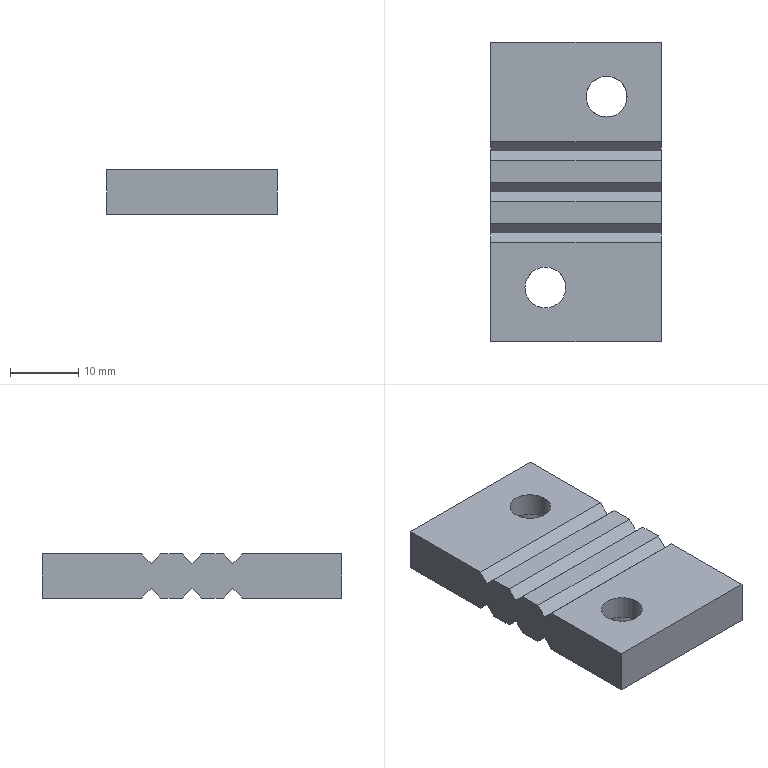Part | NX | features DATUM_CSYS 6, SKETCH 5, EXTRUDE 3, DATUM_PLANE 2, EXTRACT_STRING 2, SWP104 2, BREP 1, Instance Feature 1, Mirror Feature 1, TRIM BODY 1, UNITE 1 | 1 solid | 28 faces | box 25 x 44 x 6.5 mm | volume 6256 mm3 | plane 24 | cylinder 2 | cone 2 | commonest cylinder face diameters 6 x2
STEP:
#1=CARTESIAN_POINT('',(12.5,4.586,0.));
#2=VERTEX_POINT('',#1);
#3=CARTESIAN_POINT('',(12.5,6.,-1.414));
#4=VERTEX_POINT('',#3);
#5=CARTESIAN_POINT('',(12.5,-11.957,16.543));
#6=DIRECTION('',(0.,0.7071,-0.7071));
#7=VECTOR('',#6,1000.);
#8=LINE('',#5,#7);
#9=EDGE_CURVE('',#2,#4,#8,.T.);
#10=ORIENTED_EDGE('',*,*,#9,.F.);
#11=CARTESIAN_POINT('',(12.5,1.414,0.));
#12=VERTEX_POINT('',#11);
#13=CARTESIAN_POINT('',(12.5,-22.,0.));
#14=DIRECTION('',(0.,1.,0.));
#15=VECTOR('',#14,1000.);
#16=LINE('',#13,#15);
#17=EDGE_CURVE('',#12,#2,#16,.T.);
#18=ORIENTED_EDGE('',*,*,#17,.F.);
#19=CARTESIAN_POINT('',(12.5,0.,-1.414));
#20=VERTEX_POINT('',#19);
#21=CARTESIAN_POINT('',(12.5,-7.043,-8.457));
#22=DIRECTION('',(0.,0.7071,0.7071));
#23=VECTOR('',#22,1000.);
#24=LINE('',#21,#23);
#25=EDGE_CURVE('',#20,#12,#24,.T.);
#26=ORIENTED_EDGE('',*,*,#25,.F.);
#27=CARTESIAN_POINT('',(12.5,-1.414,0.));
#28=VERTEX_POINT('',#27);
#29=CARTESIAN_POINT('',(12.5,-14.957,13.543));
#30=DIRECTION('',(0.,0.7071,-0.7071));
#31=VECTOR('',#30,1000.);
#32=LINE('',#29,#31);
#33=EDGE_CURVE('',#28,#20,#32,.T.);
#34=ORIENTED_EDGE('',*,*,#33,.F.);
#35=CARTESIAN_POINT('',(12.5,-4.586,0.));
#36=VERTEX_POINT('',#35);
#37=CARTESIAN_POINT('',(12.5,-22.,0.));
#38=DIRECTION('',(0.,1.,0.));
#39=VECTOR('',#38,1000.);
#40=LINE('',#37,#39);
#41=EDGE_CURVE('',#36,#28,#40,.T.);
#42=ORIENTED_EDGE('',*,*,#41,.F.);
#43=CARTESIAN_POINT('',(12.5,-6.,-1.414));
#44=VERTEX_POINT('',#43);
#45=CARTESIAN_POINT('',(12.5,-10.043,-5.457));
#46=DIRECTION('',(0.,0.7071,0.7071));
#47=VECTOR('',#46,1000.);
#48=LINE('',#45,#47);
#49=EDGE_CURVE('',#44,#36,#48,.T.);
#50=ORIENTED_EDGE('',*,*,#49,.F.);
#51=CARTESIAN_POINT('',(12.5,-7.414,0.));
#52=VERTEX_POINT('',#51);
#53=CARTESIAN_POINT('',(12.5,-17.957,10.543));
#54=DIRECTION('',(0.,0.7071,-0.7071));
#55=VECTOR('',#54,1000.);
#56=LINE('',#53,#55);
#57=EDGE_CURVE('',#52,#44,#56,.T.);
#58=ORIENTED_EDGE('',*,*,#57,.F.);
#59=CARTESIAN_POINT('',(12.5,-22.,0.));
#60=VERTEX_POINT('',#59);
#61=CARTESIAN_POINT('',(12.5,-22.,0.));
#62=DIRECTION('',(0.,1.,0.));
#63=VECTOR('',#62,1000.);
#64=LINE('',#61,#63);
#65=EDGE_CURVE('',#60,#52,#64,.T.);
#66=ORIENTED_EDGE('',*,*,#65,.F.);
#67=CARTESIAN_POINT('',(12.5,-22.,-6.5));
#68=VERTEX_POINT('',#67);
#69=CARTESIAN_POINT('',(12.5,-22.,6.5));
#70=DIRECTION('',(0.,0.,-1.));
#71=VECTOR('',#70,1000.);
#72=LINE('',#69,#71);
#73=EDGE_CURVE('',#60,#68,#72,.T.);
#74=ORIENTED_EDGE('',*,*,#73,.T.);
#75=CARTESIAN_POINT('',(12.5,-7.414,-6.5));
#76=VERTEX_POINT('',#75);
#77=CARTESIAN_POINT('',(12.5,-22.,-6.5));
#78=DIRECTION('',(0.,1.,0.));
#79=VECTOR('',#78,1000.);
#80=LINE('',#77,#79);
#81=EDGE_CURVE('',#68,#76,#80,.T.);
#82=ORIENTED_EDGE('',*,*,#81,.T.);
#83=CARTESIAN_POINT('',(12.5,-6.,-5.086));
#84=VERTEX_POINT('',#83);
#85=CARTESIAN_POINT('',(12.5,-8.207,-7.293));
#86=DIRECTION('',(0.,0.7071,0.7071));
#87=VECTOR('',#86,1000.);
#88=LINE('',#85,#87);
#89=EDGE_CURVE('',#76,#84,#88,.T.);
#90=ORIENTED_EDGE('',*,*,#89,.T.);
#91=CARTESIAN_POINT('',(12.5,-4.586,-6.5));
#92=VERTEX_POINT('',#91);
#93=CARTESIAN_POINT('',(12.5,-19.793,8.707));
#94=DIRECTION('',(0.,0.7071,-0.7071));
#95=VECTOR('',#94,1000.);
#96=LINE('',#93,#95);
#97=EDGE_CURVE('',#84,#92,#96,.T.);
#98=ORIENTED_EDGE('',*,*,#97,.T.);
#99=CARTESIAN_POINT('',(12.5,-1.414,-6.5));
#100=VERTEX_POINT('',#99);
#101=CARTESIAN_POINT('',(12.5,-22.,-6.5));
#102=DIRECTION('',(0.,1.,0.));
#103=VECTOR('',#102,1000.);
#104=LINE('',#101,#103);
#105=EDGE_CURVE('',#92,#100,#104,.T.);
#106=ORIENTED_EDGE('',*,*,#105,.T.);
#107=CARTESIAN_POINT('',(12.5,0.,-5.086));
#108=VERTEX_POINT('',#107);
#109=CARTESIAN_POINT('',(12.5,-5.207,-10.293));
#110=DIRECTION('',(0.,0.7071,0.7071));
#111=VECTOR('',#110,1000.);
#112=LINE('',#109,#111);
#113=EDGE_CURVE('',#100,#108,#112,.T.);
#114=ORIENTED_EDGE('',*,*,#113,.T.);
#115=CARTESIAN_POINT('',(12.5,1.414,-6.5));
#116=VERTEX_POINT('',#115);
#117=CARTESIAN_POINT('',(12.5,-16.793,11.707));
#118=DIRECTION('',(0.,0.7071,-0.7071));
#119=VECTOR('',#118,1000.);
#120=LINE('',#117,#119);
#121=EDGE_CURVE('',#108,#116,#120,.T.);
#122=ORIENTED_EDGE('',*,*,#121,.T.);
#123=CARTESIAN_POINT('',(12.5,4.586,-6.5));
#124=VERTEX_POINT('',#123);
#125=CARTESIAN_POINT('',(12.5,-22.,-6.5));
#126=DIRECTION('',(0.,1.,0.));
#127=VECTOR('',#126,1000.);
#128=LINE('',#125,#127);
#129=EDGE_CURVE('',#116,#124,#128,.T.);
#130=ORIENTED_EDGE('',*,*,#129,.T.);
#131=CARTESIAN_POINT('',(12.5,6.,-5.086));
#132=VERTEX_POINT('',#131);
#133=CARTESIAN_POINT('',(12.5,-2.207,-13.293));
#134=DIRECTION('',(0.,0.7071,0.7071));
#135=VECTOR('',#134,1000.);
#136=LINE('',#133,#135);
#137=EDGE_CURVE('',#124,#132,#136,.T.);
#138=ORIENTED_EDGE('',*,*,#137,.T.);
#139=CARTESIAN_POINT('',(12.5,7.414,-6.5));
#140=VERTEX_POINT('',#139);
#141=CARTESIAN_POINT('',(12.5,-13.793,14.707));
#142=DIRECTION('',(0.,0.7071,-0.7071));
#143=VECTOR('',#142,1000.);
#144=LINE('',#141,#143);
#145=EDGE_CURVE('',#132,#140,#144,.T.);
#146=ORIENTED_EDGE('',*,*,#145,.T.);
#147=CARTESIAN_POINT('',(12.5,22.,-6.5));
#148=VERTEX_POINT('',#147);
#149=CARTESIAN_POINT('',(12.5,-22.,-6.5));
#150=DIRECTION('',(0.,1.,0.));
#151=VECTOR('',#150,1000.);
#152=LINE('',#149,#151);
#153=EDGE_CURVE('',#140,#148,#152,.T.);
#154=ORIENTED_EDGE('',*,*,#153,.T.);
#155=CARTESIAN_POINT('',(12.5,22.,0.));
#156=VERTEX_POINT('',#155);
#157=CARTESIAN_POINT('',(12.5,22.,6.5));
#158=DIRECTION('',(0.,0.,-1.));
#159=VECTOR('',#158,1000.);
#160=LINE('',#157,#159);
#161=EDGE_CURVE('',#156,#148,#160,.T.);
#162=ORIENTED_EDGE('',*,*,#161,.F.);
#163=CARTESIAN_POINT('',(12.5,7.414,0.));
#164=VERTEX_POINT('',#163);
#165=CARTESIAN_POINT('',(12.5,-22.,0.));
#166=DIRECTION('',(0.,1.,0.));
#167=VECTOR('',#166,1000.);
#168=LINE('',#165,#167);
#169=EDGE_CURVE('',#164,#156,#168,.T.);
#170=ORIENTED_EDGE('',*,*,#169,.F.);
#171=CARTESIAN_POINT('',(12.5,-4.043,-11.457));
#172=DIRECTION('',(0.,0.7071,0.7071));
#173=VECTOR('',#172,1000.);
#174=LINE('',#171,#173);
#175=EDGE_CURVE('',#4,#164,#174,.T.);
#176=ORIENTED_EDGE('',*,*,#175,.F.);
#177=EDGE_LOOP('',(#10,#18,#26,#34,#42,#50,#58,#66,#74,#82,#90,#98,#106,#114,#122,#130,#138,#146,#154,#162,#170,#176));
#178=FACE_BOUND('',#177,.T.);
#179=CARTESIAN_POINT('',(12.5,-22.,6.5));
#180=DIRECTION('',(-1.,0.,0.));
#181=DIRECTION('',(0.,0.,1.));
#182=AXIS2_PLACEMENT_3D('',#179,#180,#181);
#183=PLANE('',#182);
#184=ADVANCED_FACE('',(#178),#183,.F.);
#185=ORIENTED_EDGE('',*,*,#17,.T.);
#186=CARTESIAN_POINT('',(-12.5,4.586,0.));
#187=VERTEX_POINT('',#186);
#188=CARTESIAN_POINT('',(19.5,4.586,0.));
#189=DIRECTION('',(-1.,0.,0.));
#190=VECTOR('',#189,1000.);
#191=LINE('',#188,#190);
#192=EDGE_CURVE('',#2,#187,#191,.T.);
#193=ORIENTED_EDGE('',*,*,#192,.T.);
#194=CARTESIAN_POINT('',(-12.5,1.414,0.));
#195=VERTEX_POINT('',#194);
#196=CARTESIAN_POINT('',(-12.5,22.,0.));
#197=DIRECTION('',(0.,-1.,0.));
#198=VECTOR('',#197,1000.);
#199=LINE('',#196,#198);
#200=EDGE_CURVE('',#187,#195,#199,.T.);
#201=ORIENTED_EDGE('',*,*,#200,.T.);
#202=CARTESIAN_POINT('',(19.5,1.414,0.));
#203=DIRECTION('',(-1.,0.,0.));
#204=VECTOR('',#203,1000.);
#205=LINE('',#202,#204);
#206=EDGE_CURVE('',#12,#195,#205,.T.);
#207=ORIENTED_EDGE('',*,*,#206,.F.);
#208=EDGE_LOOP('',(#185,#193,#201,#207));
#209=FACE_BOUND('',#208,.T.);
#210=CARTESIAN_POINT('',(0.,0.,0.));
#211=DIRECTION('',(0.,0.,1.));
#212=DIRECTION('',(1.,0.,0.));
#213=AXIS2_PLACEMENT_3D('',#210,#211,#212);
#214=PLANE('',#213);
#215=ADVANCED_FACE('',(#209),#214,.T.);
#216=CARTESIAN_POINT('',(7.5,14.,0.));
#217=VERTEX_POINT('',#216);
#218=CARTESIAN_POINT('',(4.5,14.,0.));
#219=DIRECTION('',(0.,0.,1.));
#220=DIRECTION('',(1.,0.,0.));
#221=AXIS2_PLACEMENT_3D('',#218,#219,#220);
#222=CIRCLE('',#221,3.);
#223=EDGE_CURVE('',#217,#217,#222,.F.);
#224=ORIENTED_EDGE('',*,*,#223,.T.);
#225=EDGE_LOOP('',(#224));
#226=FACE_BOUND('',#225,.T.);
#227=CARTESIAN_POINT('',(-12.5,22.,0.));
#228=VERTEX_POINT('',#227);
#229=CARTESIAN_POINT('',(-12.5,7.414,0.));
#230=VERTEX_POINT('',#229);
#231=CARTESIAN_POINT('',(-12.5,22.,0.));
#232=DIRECTION('',(0.,-1.,0.));
#233=VECTOR('',#232,1000.);
#234=LINE('',#231,#233);
#235=EDGE_CURVE('',#228,#230,#234,.T.);
#236=ORIENTED_EDGE('',*,*,#235,.T.);
#237=CARTESIAN_POINT('',(19.5,7.414,0.));
#238=DIRECTION('',(-1.,0.,0.));
#239=VECTOR('',#238,1000.);
#240=LINE('',#237,#239);
#241=EDGE_CURVE('',#164,#230,#240,.T.);
#242=ORIENTED_EDGE('',*,*,#241,.F.);
#243=ORIENTED_EDGE('',*,*,#169,.T.);
#244=CARTESIAN_POINT('',(12.5,22.,0.));
#245=DIRECTION('',(-1.,0.,0.));
#246=VECTOR('',#245,1000.);
#247=LINE('',#244,#246);
#248=EDGE_CURVE('',#156,#228,#247,.T.);
#249=ORIENTED_EDGE('',*,*,#248,.T.);
#250=EDGE_LOOP('',(#236,#242,#243,#249));
#251=FACE_BOUND('',#250,.T.);
#252=CARTESIAN_POINT('',(0.,0.,0.));
#253=DIRECTION('',(0.,0.,1.));
#254=DIRECTION('',(1.,0.,0.));
#255=AXIS2_PLACEMENT_3D('',#252,#253,#254);
#256=PLANE('',#255);
#257=ADVANCED_FACE('',(#226,#251),#256,.T.);
#258=ORIENTED_EDGE('',*,*,#41,.T.);
#259=CARTESIAN_POINT('',(-12.5,-1.414,0.));
#260=VERTEX_POINT('',#259);
#261=CARTESIAN_POINT('',(19.5,-1.414,0.));
#262=DIRECTION('',(-1.,0.,0.));
#263=VECTOR('',#262,1000.);
#264=LINE('',#261,#263);
#265=EDGE_CURVE('',#28,#260,#264,.T.);
#266=ORIENTED_EDGE('',*,*,#265,.T.);
#267=CARTESIAN_POINT('',(-12.5,-4.586,0.));
#268=VERTEX_POINT('',#267);
#269=CARTESIAN_POINT('',(-12.5,22.,0.));
#270=DIRECTION('',(0.,-1.,0.));
#271=VECTOR('',#270,1000.);
#272=LINE('',#269,#271);
#273=EDGE_CURVE('',#260,#268,#272,.T.);
#274=ORIENTED_EDGE('',*,*,#273,.T.);
#275=CARTESIAN_POINT('',(19.5,-4.586,0.));
#276=DIRECTION('',(-1.,0.,0.));
#277=VECTOR('',#276,1000.);
#278=LINE('',#275,#277);
#279=EDGE_CURVE('',#36,#268,#278,.T.);
#280=ORIENTED_EDGE('',*,*,#279,.F.);
#281=EDGE_LOOP('',(#258,#266,#274,#280));
#282=FACE_BOUND('',#281,.T.);
#283=CARTESIAN_POINT('',(0.,0.,0.));
#284=DIRECTION('',(0.,0.,1.));
#285=DIRECTION('',(1.,0.,0.));
#286=AXIS2_PLACEMENT_3D('',#283,#284,#285);
#287=PLANE('',#286);
#288=ADVANCED_FACE('',(#282),#287,.T.);
#289=CARTESIAN_POINT('',(-1.5,-14.043,0.));
#290=VERTEX_POINT('',#289);
#291=CARTESIAN_POINT('',(-4.5,-14.043,0.));
#292=DIRECTION('',(0.,0.,1.));
#293=DIRECTION('',(1.,0.,0.));
#294=AXIS2_PLACEMENT_3D('',#291,#292,#293);
#295=CIRCLE('',#294,3.);
#296=EDGE_CURVE('',#290,#290,#295,.T.);
#297=ORIENTED_EDGE('',*,*,#296,.F.);
#298=EDGE_LOOP('',(#297));
#299=FACE_BOUND('',#298,.T.);
#300=ORIENTED_EDGE('',*,*,#65,.T.);
#301=CARTESIAN_POINT('',(-12.5,-7.414,0.));
#302=VERTEX_POINT('',#301);
#303=CARTESIAN_POINT('',(19.5,-7.414,0.));
#304=DIRECTION('',(-1.,0.,0.));
#305=VECTOR('',#304,1000.);
#306=LINE('',#303,#305);
#307=EDGE_CURVE('',#52,#302,#306,.T.);
#308=ORIENTED_EDGE('',*,*,#307,.T.);
#309=CARTESIAN_POINT('',(-12.5,-22.,0.));
#310=VERTEX_POINT('',#309);
#311=CARTESIAN_POINT('',(-12.5,22.,0.));
#312=DIRECTION('',(0.,-1.,0.));
#313=VECTOR('',#312,1000.);
#314=LINE('',#311,#313);
#315=EDGE_CURVE('',#302,#310,#314,.T.);
#316=ORIENTED_EDGE('',*,*,#315,.T.);
#317=CARTESIAN_POINT('',(-12.5,-22.,0.));
#318=DIRECTION('',(1.,0.,0.));
#319=VECTOR('',#318,1000.);
#320=LINE('',#317,#319);
#321=EDGE_CURVE('',#310,#60,#320,.T.);
#322=ORIENTED_EDGE('',*,*,#321,.T.);
#323=EDGE_LOOP('',(#300,#308,#316,#322));
#324=FACE_BOUND('',#323,.T.);
#325=CARTESIAN_POINT('',(0.,0.,0.));
#326=DIRECTION('',(0.,0.,1.));
#327=DIRECTION('',(1.,0.,0.));
#328=AXIS2_PLACEMENT_3D('',#325,#326,#327);
#329=PLANE('',#328);
#330=ADVANCED_FACE('',(#299,#324),#329,.T.);
#331=CARTESIAN_POINT('',(-12.5,6.,-1.414));
#332=VERTEX_POINT('',#331);
#333=CARTESIAN_POINT('',(-12.5,4.586,0.));
#334=DIRECTION('',(0.,0.7071,-0.7071));
#335=VECTOR('',#334,1000.);
#336=LINE('',#333,#335);
#337=EDGE_CURVE('',#187,#332,#336,.T.);
#338=ORIENTED_EDGE('',*,*,#337,.T.);
#339=CARTESIAN_POINT('',(-12.5,6.,-1.414));
#340=DIRECTION('',(0.,0.7071,0.7071));
#341=VECTOR('',#340,1000.);
#342=LINE('',#339,#341);
#343=EDGE_CURVE('',#332,#230,#342,.T.);
#344=ORIENTED_EDGE('',*,*,#343,.T.);
#345=ORIENTED_EDGE('',*,*,#235,.F.);
#346=CARTESIAN_POINT('',(-12.5,22.,-6.5));
#347=VERTEX_POINT('',#346);
#348=CARTESIAN_POINT('',(-12.5,22.,6.5));
#349=DIRECTION('',(0.,0.,-1.));
#350=VECTOR('',#349,1000.);
#351=LINE('',#348,#350);
#352=EDGE_CURVE('',#228,#347,#351,.T.);
#353=ORIENTED_EDGE('',*,*,#352,.T.);
#354=CARTESIAN_POINT('',(-12.5,7.414,-6.5));
#355=VERTEX_POINT('',#354);
#356=CARTESIAN_POINT('',(-12.5,22.,-6.5));
#357=DIRECTION('',(0.,-1.,0.));
#358=VECTOR('',#357,1000.);
#359=LINE('',#356,#358);
#360=EDGE_CURVE('',#347,#355,#359,.T.);
#361=ORIENTED_EDGE('',*,*,#360,.T.);
#362=CARTESIAN_POINT('',(-12.5,6.,-5.086));
#363=VERTEX_POINT('',#362);
#364=CARTESIAN_POINT('',(-12.5,6.,-5.086));
#365=DIRECTION('',(0.,0.7071,-0.7071));
#366=VECTOR('',#365,1000.);
#367=LINE('',#364,#366);
#368=EDGE_CURVE('',#363,#355,#367,.T.);
#369=ORIENTED_EDGE('',*,*,#368,.F.);
#370=CARTESIAN_POINT('',(-12.5,4.586,-6.5));
#371=VERTEX_POINT('',#370);
#372=CARTESIAN_POINT('',(-12.5,4.586,-6.5));
#373=DIRECTION('',(0.,0.7071,0.7071));
#374=VECTOR('',#373,1000.);
#375=LINE('',#372,#374);
#376=EDGE_CURVE('',#371,#363,#375,.T.);
#377=ORIENTED_EDGE('',*,*,#376,.F.);
#378=CARTESIAN_POINT('',(-12.5,1.414,-6.5));
#379=VERTEX_POINT('',#378);
#380=CARTESIAN_POINT('',(-12.5,22.,-6.5));
#381=DIRECTION('',(0.,-1.,0.));
#382=VECTOR('',#381,1000.);
#383=LINE('',#380,#382);
#384=EDGE_CURVE('',#371,#379,#383,.T.);
#385=ORIENTED_EDGE('',*,*,#384,.T.);
#386=CARTESIAN_POINT('',(-12.5,0.,-5.086));
#387=VERTEX_POINT('',#386);
#388=CARTESIAN_POINT('',(-12.5,0.,-5.086));
#389=DIRECTION('',(0.,0.7071,-0.7071));
#390=VECTOR('',#389,1000.);
#391=LINE('',#388,#390);
#392=EDGE_CURVE('',#387,#379,#391,.T.);
#393=ORIENTED_EDGE('',*,*,#392,.F.);
#394=CARTESIAN_POINT('',(-12.5,-1.414,-6.5));
#395=VERTEX_POINT('',#394);
#396=CARTESIAN_POINT('',(-12.5,-1.414,-6.5));
#397=DIRECTION('',(0.,0.7071,0.7071));
#398=VECTOR('',#397,1000.);
#399=LINE('',#396,#398);
#400=EDGE_CURVE('',#395,#387,#399,.T.);
#401=ORIENTED_EDGE('',*,*,#400,.F.);
#402=CARTESIAN_POINT('',(-12.5,-4.586,-6.5));
#403=VERTEX_POINT('',#402);
#404=CARTESIAN_POINT('',(-12.5,22.,-6.5));
#405=DIRECTION('',(0.,-1.,0.));
#406=VECTOR('',#405,1000.);
#407=LINE('',#404,#406);
#408=EDGE_CURVE('',#395,#403,#407,.T.);
#409=ORIENTED_EDGE('',*,*,#408,.T.);
#410=CARTESIAN_POINT('',(-12.5,-6.,-5.086));
#411=VERTEX_POINT('',#410);
#412=CARTESIAN_POINT('',(-12.5,-6.,-5.086));
#413=DIRECTION('',(0.,0.7071,-0.7071));
#414=VECTOR('',#413,1000.);
#415=LINE('',#412,#414);
#416=EDGE_CURVE('',#411,#403,#415,.T.);
#417=ORIENTED_EDGE('',*,*,#416,.F.);
#418=CARTESIAN_POINT('',(-12.5,-7.414,-6.5));
#419=VERTEX_POINT('',#418);
#420=CARTESIAN_POINT('',(-12.5,-7.414,-6.5));
#421=DIRECTION('',(0.,0.7071,0.7071));
#422=VECTOR('',#421,1000.);
#423=LINE('',#420,#422);
#424=EDGE_CURVE('',#419,#411,#423,.T.);
#425=ORIENTED_EDGE('',*,*,#424,.F.);
#426=CARTESIAN_POINT('',(-12.5,-22.,-6.5));
#427=VERTEX_POINT('',#426);
#428=CARTESIAN_POINT('',(-12.5,22.,-6.5));
#429=DIRECTION('',(0.,-1.,0.));
#430=VECTOR('',#429,1000.);
#431=LINE('',#428,#430);
#432=EDGE_CURVE('',#419,#427,#431,.T.);
#433=ORIENTED_EDGE('',*,*,#432,.T.);
#434=CARTESIAN_POINT('',(-12.5,-22.,6.5));
#435=DIRECTION('',(0.,0.,-1.));
#436=VECTOR('',#435,1000.);
#437=LINE('',#434,#436);
#438=EDGE_CURVE('',#310,#427,#437,.T.);
#439=ORIENTED_EDGE('',*,*,#438,.F.);
#440=ORIENTED_EDGE('',*,*,#315,.F.);
#441=CARTESIAN_POINT('',(-12.5,-6.,-1.414));
#442=VERTEX_POINT('',#441);
#443=CARTESIAN_POINT('',(-12.5,-7.414,0.));
#444=DIRECTION('',(0.,0.7071,-0.7071));
#445=VECTOR('',#444,1000.);
#446=LINE('',#443,#445);
#447=EDGE_CURVE('',#302,#442,#446,.T.);
#448=ORIENTED_EDGE('',*,*,#447,.T.);
#449=CARTESIAN_POINT('',(-12.5,-6.,-1.414));
#450=DIRECTION('',(0.,0.7071,0.7071));
#451=VECTOR('',#450,1000.);
#452=LINE('',#449,#451);
#453=EDGE_CURVE('',#442,#268,#452,.T.);
#454=ORIENTED_EDGE('',*,*,#453,.T.);
#455=ORIENTED_EDGE('',*,*,#273,.F.);
#456=CARTESIAN_POINT('',(-12.5,0.,-1.414));
#457=VERTEX_POINT('',#456);
#458=CARTESIAN_POINT('',(-12.5,-1.414,0.));
#459=DIRECTION('',(0.,0.7071,-0.7071));
#460=VECTOR('',#459,1000.);
#461=LINE('',#458,#460);
#462=EDGE_CURVE('',#260,#457,#461,.T.);
#463=ORIENTED_EDGE('',*,*,#462,.T.);
#464=CARTESIAN_POINT('',(-12.5,0.,-1.414));
#465=DIRECTION('',(0.,0.7071,0.7071));
#466=VECTOR('',#465,1000.);
#467=LINE('',#464,#466);
#468=EDGE_CURVE('',#457,#195,#467,.T.);
#469=ORIENTED_EDGE('',*,*,#468,.T.);
#470=ORIENTED_EDGE('',*,*,#200,.F.);
#471=EDGE_LOOP('',(#338,#344,#345,#353,#361,#369,#377,#385,#393,#401,#409,#417,#425,#433,#439,#440,#448,#454,#455,#463,#469,#470));
#472=FACE_BOUND('',#471,.T.);
#473=CARTESIAN_POINT('',(-12.5,22.,6.5));
#474=DIRECTION('',(1.,0.,0.));
#475=DIRECTION('',(0.,0.,-1.));
#476=AXIS2_PLACEMENT_3D('',#473,#474,#475);
#477=PLANE('',#476);
#478=ADVANCED_FACE('',(#472),#477,.F.);
#479=CARTESIAN_POINT('',(19.5,-7.414,-6.5));
#480=DIRECTION('',(-1.,0.,0.));
#481=VECTOR('',#480,1000.);
#482=LINE('',#479,#481);
#483=EDGE_CURVE('',#76,#419,#482,.T.);
#484=ORIENTED_EDGE('',*,*,#483,.F.);
#485=ORIENTED_EDGE('',*,*,#81,.F.);
#486=CARTESIAN_POINT('',(-12.5,-22.,-6.5));
#487=DIRECTION('',(1.,0.,0.));
#488=VECTOR('',#487,1000.);
#489=LINE('',#486,#488);
#490=EDGE_CURVE('',#427,#68,#489,.T.);
#491=ORIENTED_EDGE('',*,*,#490,.F.);
#492=ORIENTED_EDGE('',*,*,#432,.F.);
#493=EDGE_LOOP('',(#484,#485,#491,#492));
#494=FACE_BOUND('',#493,.T.);
#495=CARTESIAN_POINT('',(-10.5,-14.043,-6.5));
#496=VERTEX_POINT('',#495);
#497=CARTESIAN_POINT('',(-4.5,-14.043,-6.5));
#498=DIRECTION('',(0.,0.,-1.));
#499=DIRECTION('',(-1.,0.,0.));
#500=AXIS2_PLACEMENT_3D('',#497,#498,#499);
#501=CIRCLE('',#500,6.);
#502=EDGE_CURVE('',#496,#496,#501,.T.);
#503=ORIENTED_EDGE('',*,*,#502,.F.);
#504=EDGE_LOOP('',(#503));
#505=FACE_BOUND('',#504,.T.);
#506=CARTESIAN_POINT('',(0.,0.,-6.5));
#507=DIRECTION('',(0.,0.,-1.));
#508=DIRECTION('',(1.,0.,0.));
#509=AXIS2_PLACEMENT_3D('',#506,#507,#508);
#510=PLANE('',#509);
#511=ADVANCED_FACE('',(#494,#505),#510,.T.);
#512=CARTESIAN_POINT('',(19.5,-4.586,-6.5));
#513=DIRECTION('',(-1.,0.,0.));
#514=VECTOR('',#513,1000.);
#515=LINE('',#512,#514);
#516=EDGE_CURVE('',#92,#403,#515,.T.);
#517=ORIENTED_EDGE('',*,*,#516,.T.);
#518=ORIENTED_EDGE('',*,*,#408,.F.);
#519=CARTESIAN_POINT('',(19.5,-1.414,-6.5));
#520=DIRECTION('',(-1.,0.,0.));
#521=VECTOR('',#520,1000.);
#522=LINE('',#519,#521);
#523=EDGE_CURVE('',#100,#395,#522,.T.);
#524=ORIENTED_EDGE('',*,*,#523,.F.);
#525=ORIENTED_EDGE('',*,*,#105,.F.);
#526=EDGE_LOOP('',(#517,#518,#524,#525));
#527=FACE_BOUND('',#526,.T.);
#528=CARTESIAN_POINT('',(0.,0.,-6.5));
#529=DIRECTION('',(0.,0.,-1.));
#530=DIRECTION('',(1.,0.,0.));
#531=AXIS2_PLACEMENT_3D('',#528,#529,#530);
#532=PLANE('',#531);
#533=ADVANCED_FACE('',(#527),#532,.T.);
#534=CARTESIAN_POINT('',(19.5,1.414,-6.5));
#535=DIRECTION('',(-1.,0.,0.));
#536=VECTOR('',#535,1000.);
#537=LINE('',#534,#536);
#538=EDGE_CURVE('',#116,#379,#537,.T.);
#539=ORIENTED_EDGE('',*,*,#538,.T.);
#540=ORIENTED_EDGE('',*,*,#384,.F.);
#541=CARTESIAN_POINT('',(19.5,4.586,-6.5));
#542=DIRECTION('',(-1.,0.,0.));
#543=VECTOR('',#542,1000.);
#544=LINE('',#541,#543);
#545=EDGE_CURVE('',#124,#371,#544,.T.);
#546=ORIENTED_EDGE('',*,*,#545,.F.);
#547=ORIENTED_EDGE('',*,*,#129,.F.);
#548=EDGE_LOOP('',(#539,#540,#546,#547));
#549=FACE_BOUND('',#548,.T.);
#550=CARTESIAN_POINT('',(0.,0.,-6.5));
#551=DIRECTION('',(0.,0.,-1.));
#552=DIRECTION('',(1.,0.,0.));
#553=AXIS2_PLACEMENT_3D('',#550,#551,#552);
#554=PLANE('',#553);
#555=ADVANCED_FACE('',(#549),#554,.T.);
#556=ORIENTED_EDGE('',*,*,#248,.F.);
#557=ORIENTED_EDGE('',*,*,#161,.T.);
#558=CARTESIAN_POINT('',(12.5,22.,-6.5));
#559=DIRECTION('',(-1.,0.,0.));
#560=VECTOR('',#559,1000.);
#561=LINE('',#558,#560);
#562=EDGE_CURVE('',#148,#347,#561,.T.);
#563=ORIENTED_EDGE('',*,*,#562,.T.);
#564=ORIENTED_EDGE('',*,*,#352,.F.);
#565=EDGE_LOOP('',(#556,#557,#563,#564));
#566=FACE_BOUND('',#565,.T.);
#567=CARTESIAN_POINT('',(12.5,22.,6.5));
#568=DIRECTION('',(0.,-1.,0.));
#569=DIRECTION('',(0.,0.,-1.));
#570=AXIS2_PLACEMENT_3D('',#567,#568,#569);
#571=PLANE('',#570);
#572=ADVANCED_FACE('',(#566),#571,.F.);
#573=ORIENTED_EDGE('',*,*,#321,.F.);
#574=ORIENTED_EDGE('',*,*,#438,.T.);
#575=ORIENTED_EDGE('',*,*,#490,.T.);
#576=ORIENTED_EDGE('',*,*,#73,.F.);
#577=EDGE_LOOP('',(#573,#574,#575,#576));
#578=FACE_BOUND('',#577,.T.);
#579=CARTESIAN_POINT('',(-12.5,-22.,6.5));
#580=DIRECTION('',(0.,1.,0.));
#581=DIRECTION('',(0.,0.,1.));
#582=AXIS2_PLACEMENT_3D('',#579,#580,#581);
#583=PLANE('',#582);
#584=ADVANCED_FACE('',(#578),#583,.F.);
#585=CARTESIAN_POINT('',(4.5,11.,-3.5));
#586=VERTEX_POINT('',#585);
#587=CARTESIAN_POINT('',(4.5,14.,-3.5));
#588=DIRECTION('',(0.,0.,1.));
#589=DIRECTION('',(0.,-1.,0.));
#590=AXIS2_PLACEMENT_3D('',#587,#588,#589);
#591=CIRCLE('',#590,3.);
#592=EDGE_CURVE('',#586,#586,#591,.F.);
#593=ORIENTED_EDGE('',*,*,#592,.T.);
#594=EDGE_LOOP('',(#593));
#595=FACE_BOUND('',#594,.T.);
#596=ORIENTED_EDGE('',*,*,#223,.F.);
#597=EDGE_LOOP('',(#596));
#598=FACE_BOUND('',#597,.T.);
#599=CARTESIAN_POINT('',(4.5,14.,6.5));
#600=DIRECTION('',(0.,0.,1.));
#601=DIRECTION('',(0.,-1.,0.));
#602=AXIS2_PLACEMENT_3D('',#599,#600,#601);
#603=CYLINDRICAL_SURFACE('',#602,3.);
#604=ADVANCED_FACE('',(#595,#598),#603,.F.);
#605=CARTESIAN_POINT('',(-7.5,-14.043,-3.5));
#606=VERTEX_POINT('',#605);
#607=CARTESIAN_POINT('',(-4.5,-14.043,-3.5));
#608=DIRECTION('',(0.,0.,-1.));
#609=DIRECTION('',(-1.,0.,0.));
#610=AXIS2_PLACEMENT_3D('',#607,#608,#609);
#611=CIRCLE('',#610,3.);
#612=EDGE_CURVE('',#606,#606,#611,.F.);
#613=ORIENTED_EDGE('',*,*,#612,.F.);
#614=EDGE_LOOP('',(#613));
#615=FACE_BOUND('',#614,.T.);
#616=ORIENTED_EDGE('',*,*,#296,.T.);
#617=EDGE_LOOP('',(#616));
#618=FACE_BOUND('',#617,.T.);
#619=CARTESIAN_POINT('',(-4.5,-14.043,-4.1));
#620=DIRECTION('',(0.,0.,-1.));
#621=DIRECTION('',(-1.,0.,0.));
#622=AXIS2_PLACEMENT_3D('',#619,#620,#621);
#623=CYLINDRICAL_SURFACE('',#622,3.);
#624=ADVANCED_FACE('',(#615,#618),#623,.F.);
#625=CARTESIAN_POINT('',(19.5,7.414,-6.5));
#626=DIRECTION('',(-1.,0.,0.));
#627=VECTOR('',#626,1000.);
#628=LINE('',#625,#627);
#629=EDGE_CURVE('',#140,#355,#628,.T.);
#630=ORIENTED_EDGE('',*,*,#629,.T.);
#631=ORIENTED_EDGE('',*,*,#360,.F.);
#632=ORIENTED_EDGE('',*,*,#562,.F.);
#633=ORIENTED_EDGE('',*,*,#153,.F.);
#634=EDGE_LOOP('',(#630,#631,#632,#633));
#635=FACE_BOUND('',#634,.T.);
#636=CARTESIAN_POINT('',(4.5,8.,-6.5));
#637=VERTEX_POINT('',#636);
#638=CARTESIAN_POINT('',(4.5,14.,-6.5));
#639=DIRECTION('',(0.,0.,1.));
#640=DIRECTION('',(0.,-1.,0.));
#641=AXIS2_PLACEMENT_3D('',#638,#639,#640);
#642=CIRCLE('',#641,6.);
#643=EDGE_CURVE('',#637,#637,#642,.T.);
#644=ORIENTED_EDGE('',*,*,#643,.T.);
#645=EDGE_LOOP('',(#644));
#646=FACE_BOUND('',#645,.T.);
#647=CARTESIAN_POINT('',(0.,0.,-6.5));
#648=DIRECTION('',(0.,0.,-1.));
#649=DIRECTION('',(1.,0.,0.));
#650=AXIS2_PLACEMENT_3D('',#647,#648,#649);
#651=PLANE('',#650);
#652=ADVANCED_FACE('',(#635,#646),#651,.T.);
#653=ORIENTED_EDGE('',*,*,#592,.F.);
#654=EDGE_LOOP('',(#653));
#655=FACE_BOUND('',#654,.T.);
#656=ORIENTED_EDGE('',*,*,#643,.F.);
#657=EDGE_LOOP('',(#656));
#658=FACE_BOUND('',#657,.T.);
#659=CARTESIAN_POINT('',(4.5,14.,-6.5));
#660=DIRECTION('',(0.,0.,-1.));
#661=DIRECTION('',(0.,-1.,0.));
#662=AXIS2_PLACEMENT_3D('',#659,#660,#661);
#663=CONICAL_SURFACE('',#662,6.,0.7854);
#664=ADVANCED_FACE('',(#655,#658),#663,.F.);
#665=ORIENTED_EDGE('',*,*,#612,.T.);
#666=EDGE_LOOP('',(#665));
#667=FACE_BOUND('',#666,.T.);
#668=ORIENTED_EDGE('',*,*,#502,.T.);
#669=EDGE_LOOP('',(#668));
#670=FACE_BOUND('',#669,.T.);
#671=CARTESIAN_POINT('',(-4.5,-14.043,-6.5));
#672=DIRECTION('',(0.,0.,-1.));
#673=DIRECTION('',(1.,0.,0.));
#674=AXIS2_PLACEMENT_3D('',#671,#672,#673);
#675=CONICAL_SURFACE('',#674,6.,0.7854);
#676=ADVANCED_FACE('',(#667,#670),#675,.F.);
#677=ORIENTED_EDGE('',*,*,#545,.T.);
#678=ORIENTED_EDGE('',*,*,#376,.T.);
#679=CARTESIAN_POINT('',(19.5,6.,-5.086));
#680=DIRECTION('',(-1.,0.,0.));
#681=VECTOR('',#680,1000.);
#682=LINE('',#679,#681);
#683=EDGE_CURVE('',#363,#132,#682,.F.);
#684=ORIENTED_EDGE('',*,*,#683,.T.);
#685=ORIENTED_EDGE('',*,*,#137,.F.);
#686=EDGE_LOOP('',(#677,#678,#684,#685));
#687=FACE_BOUND('',#686,.T.);
#688=CARTESIAN_POINT('',(19.5,4.586,-6.5));
#689=DIRECTION('',(0.,-0.7071,0.7071));
#690=DIRECTION('',(0.,-0.7071,-0.7071));
#691=AXIS2_PLACEMENT_3D('',#688,#689,#690);
#692=PLANE('',#691);
#693=ADVANCED_FACE('',(#687),#692,.F.);
#694=ORIENTED_EDGE('',*,*,#683,.F.);
#695=ORIENTED_EDGE('',*,*,#368,.T.);
#696=ORIENTED_EDGE('',*,*,#629,.F.);
#697=ORIENTED_EDGE('',*,*,#145,.F.);
#698=EDGE_LOOP('',(#694,#695,#696,#697));
#699=FACE_BOUND('',#698,.T.);
#700=CARTESIAN_POINT('',(19.5,6.,-5.086));
#701=DIRECTION('',(0.,0.7071,0.7071));
#702=DIRECTION('',(0.,-0.7071,0.7071));
#703=AXIS2_PLACEMENT_3D('',#700,#701,#702);
#704=PLANE('',#703);
#705=ADVANCED_FACE('',(#699),#704,.F.);
#706=ORIENTED_EDGE('',*,*,#523,.T.);
#707=ORIENTED_EDGE('',*,*,#400,.T.);
#708=CARTESIAN_POINT('',(19.5,0.,-5.086));
#709=DIRECTION('',(-1.,0.,0.));
#710=VECTOR('',#709,1000.);
#711=LINE('',#708,#710);
#712=EDGE_CURVE('',#387,#108,#711,.F.);
#713=ORIENTED_EDGE('',*,*,#712,.T.);
#714=ORIENTED_EDGE('',*,*,#113,.F.);
#715=EDGE_LOOP('',(#706,#707,#713,#714));
#716=FACE_BOUND('',#715,.T.);
#717=CARTESIAN_POINT('',(19.5,-1.414,-6.5));
#718=DIRECTION('',(0.,-0.7071,0.7071));
#719=DIRECTION('',(0.,-0.7071,-0.7071));
#720=AXIS2_PLACEMENT_3D('',#717,#718,#719);
#721=PLANE('',#720);
#722=ADVANCED_FACE('',(#716),#721,.F.);
#723=ORIENTED_EDGE('',*,*,#712,.F.);
#724=ORIENTED_EDGE('',*,*,#392,.T.);
#725=ORIENTED_EDGE('',*,*,#538,.F.);
#726=ORIENTED_EDGE('',*,*,#121,.F.);
#727=EDGE_LOOP('',(#723,#724,#725,#726));
#728=FACE_BOUND('',#727,.T.);
#729=CARTESIAN_POINT('',(19.5,0.,-5.086));
#730=DIRECTION('',(0.,0.7071,0.7071));
#731=DIRECTION('',(0.,-0.7071,0.7071));
#732=AXIS2_PLACEMENT_3D('',#729,#730,#731);
#733=PLANE('',#732);
#734=ADVANCED_FACE('',(#728),#733,.F.);
#735=ORIENTED_EDGE('',*,*,#483,.T.);
#736=ORIENTED_EDGE('',*,*,#424,.T.);
#737=CARTESIAN_POINT('',(19.5,-6.,-5.086));
#738=DIRECTION('',(-1.,0.,0.));
#739=VECTOR('',#738,1000.);
#740=LINE('',#737,#739);
#741=EDGE_CURVE('',#411,#84,#740,.F.);
#742=ORIENTED_EDGE('',*,*,#741,.T.);
#743=ORIENTED_EDGE('',*,*,#89,.F.);
#744=EDGE_LOOP('',(#735,#736,#742,#743));
#745=FACE_BOUND('',#744,.T.);
#746=CARTESIAN_POINT('',(19.5,-7.414,-6.5));
#747=DIRECTION('',(0.,-0.7071,0.7071));
#748=DIRECTION('',(0.,-0.7071,-0.7071));
#749=AXIS2_PLACEMENT_3D('',#746,#747,#748);
#750=PLANE('',#749);
#751=ADVANCED_FACE('',(#745),#750,.F.);
#752=ORIENTED_EDGE('',*,*,#741,.F.);
#753=ORIENTED_EDGE('',*,*,#416,.T.);
#754=ORIENTED_EDGE('',*,*,#516,.F.);
#755=ORIENTED_EDGE('',*,*,#97,.F.);
#756=EDGE_LOOP('',(#752,#753,#754,#755));
#757=FACE_BOUND('',#756,.T.);
#758=CARTESIAN_POINT('',(19.5,-6.,-5.086));
#759=DIRECTION('',(0.,0.7071,0.7071));
#760=DIRECTION('',(0.,-0.7071,0.7071));
#761=AXIS2_PLACEMENT_3D('',#758,#759,#760);
#762=PLANE('',#761);
#763=ADVANCED_FACE('',(#757),#762,.F.);
#764=ORIENTED_EDGE('',*,*,#57,.T.);
#765=CARTESIAN_POINT('',(19.5,-6.,-1.414));
#766=DIRECTION('',(-1.,0.,0.));
#767=VECTOR('',#766,1000.);
#768=LINE('',#765,#767);
#769=EDGE_CURVE('',#442,#44,#768,.F.);
#770=ORIENTED_EDGE('',*,*,#769,.F.);
#771=ORIENTED_EDGE('',*,*,#447,.F.);
#772=ORIENTED_EDGE('',*,*,#307,.F.);
#773=EDGE_LOOP('',(#764,#770,#771,#772));
#774=FACE_BOUND('',#773,.T.);
#775=CARTESIAN_POINT('',(19.5,-7.414,0.));
#776=DIRECTION('',(0.,0.7071,0.7071));
#777=DIRECTION('',(0.,-0.7071,0.7071));
#778=AXIS2_PLACEMENT_3D('',#775,#776,#777);
#779=PLANE('',#778);
#780=ADVANCED_FACE('',(#774),#779,.T.);
#781=ORIENTED_EDGE('',*,*,#49,.T.);
#782=ORIENTED_EDGE('',*,*,#279,.T.);
#783=ORIENTED_EDGE('',*,*,#453,.F.);
#784=ORIENTED_EDGE('',*,*,#769,.T.);
#785=EDGE_LOOP('',(#781,#782,#783,#784));
#786=FACE_BOUND('',#785,.T.);
#787=CARTESIAN_POINT('',(19.5,-6.,-1.414));
#788=DIRECTION('',(0.,-0.7071,0.7071));
#789=DIRECTION('',(0.,-0.7071,-0.7071));
#790=AXIS2_PLACEMENT_3D('',#787,#788,#789);
#791=PLANE('',#790);
#792=ADVANCED_FACE('',(#786),#791,.T.);
#793=ORIENTED_EDGE('',*,*,#33,.T.);
#794=CARTESIAN_POINT('',(19.5,0.,-1.414));
#795=DIRECTION('',(-1.,0.,0.));
#796=VECTOR('',#795,1000.);
#797=LINE('',#794,#796);
#798=EDGE_CURVE('',#457,#20,#797,.F.);
#799=ORIENTED_EDGE('',*,*,#798,.F.);
#800=ORIENTED_EDGE('',*,*,#462,.F.);
#801=ORIENTED_EDGE('',*,*,#265,.F.);
#802=EDGE_LOOP('',(#793,#799,#800,#801));
#803=FACE_BOUND('',#802,.T.);
#804=CARTESIAN_POINT('',(19.5,-1.414,0.));
#805=DIRECTION('',(0.,0.7071,0.7071));
#806=DIRECTION('',(0.,-0.7071,0.7071));
#807=AXIS2_PLACEMENT_3D('',#804,#805,#806);
#808=PLANE('',#807);
#809=ADVANCED_FACE('',(#803),#808,.T.);
#810=ORIENTED_EDGE('',*,*,#25,.T.);
#811=ORIENTED_EDGE('',*,*,#206,.T.);
#812=ORIENTED_EDGE('',*,*,#468,.F.);
#813=ORIENTED_EDGE('',*,*,#798,.T.);
#814=EDGE_LOOP('',(#810,#811,#812,#813));
#815=FACE_BOUND('',#814,.T.);
#816=CARTESIAN_POINT('',(19.5,0.,-1.414));
#817=DIRECTION('',(0.,-0.7071,0.7071));
#818=DIRECTION('',(0.,-0.7071,-0.7071));
#819=AXIS2_PLACEMENT_3D('',#816,#817,#818);
#820=PLANE('',#819);
#821=ADVANCED_FACE('',(#815),#820,.T.);
#822=ORIENTED_EDGE('',*,*,#9,.T.);
#823=CARTESIAN_POINT('',(19.5,6.,-1.414));
#824=DIRECTION('',(-1.,0.,0.));
#825=VECTOR('',#824,1000.);
#826=LINE('',#823,#825);
#827=EDGE_CURVE('',#332,#4,#826,.F.);
#828=ORIENTED_EDGE('',*,*,#827,.F.);
#829=ORIENTED_EDGE('',*,*,#337,.F.);
#830=ORIENTED_EDGE('',*,*,#192,.F.);
#831=EDGE_LOOP('',(#822,#828,#829,#830));
#832=FACE_BOUND('',#831,.T.);
#833=CARTESIAN_POINT('',(19.5,4.586,0.));
#834=DIRECTION('',(0.,0.7071,0.7071));
#835=DIRECTION('',(0.,-0.7071,0.7071));
#836=AXIS2_PLACEMENT_3D('',#833,#834,#835);
#837=PLANE('',#836);
#838=ADVANCED_FACE('',(#832),#837,.T.);
#839=ORIENTED_EDGE('',*,*,#175,.T.);
#840=ORIENTED_EDGE('',*,*,#241,.T.);
#841=ORIENTED_EDGE('',*,*,#343,.F.);
#842=ORIENTED_EDGE('',*,*,#827,.T.);
#843=EDGE_LOOP('',(#839,#840,#841,#842));
#844=FACE_BOUND('',#843,.T.);
#845=CARTESIAN_POINT('',(19.5,6.,-1.414));
#846=DIRECTION('',(0.,-0.7071,0.7071));
#847=DIRECTION('',(0.,-0.7071,-0.7071));
#848=AXIS2_PLACEMENT_3D('',#845,#846,#847);
#849=PLANE('',#848);
#850=ADVANCED_FACE('',(#844),#849,.T.);
#851=CLOSED_SHELL('',(#184,#215,#257,#288,#330,#478,#511,#533,#555,#572,#584,#604,#624,#652,#664,#676,#693,#705,#722,#734,#751,#763,#780,#792,#809,#821,#838,#850));
#852=MANIFOLD_SOLID_BREP('',#851);
#853=(LENGTH_UNIT()NAMED_UNIT(*)SI_UNIT(.MILLI.,.METRE.));
#854=UNCERTAINTY_MEASURE_WITH_UNIT(LENGTH_MEASURE(0.00001),#853,'','');
#855=(NAMED_UNIT(*)PLANE_ANGLE_UNIT()SI_UNIT($,.RADIAN.));
#856=(NAMED_UNIT(*)SI_UNIT($,.STERADIAN.)SOLID_ANGLE_UNIT());
#857=(GEOMETRIC_REPRESENTATION_CONTEXT(3)GLOBAL_UNCERTAINTY_ASSIGNED_CONTEXT((#854))GLOBAL_UNIT_ASSIGNED_CONTEXT((#853,#855,#856))REPRESENTATION_CONTEXT('',''));
#858=ADVANCED_BREP_SHAPE_REPRESENTATION('',(#852),#857);